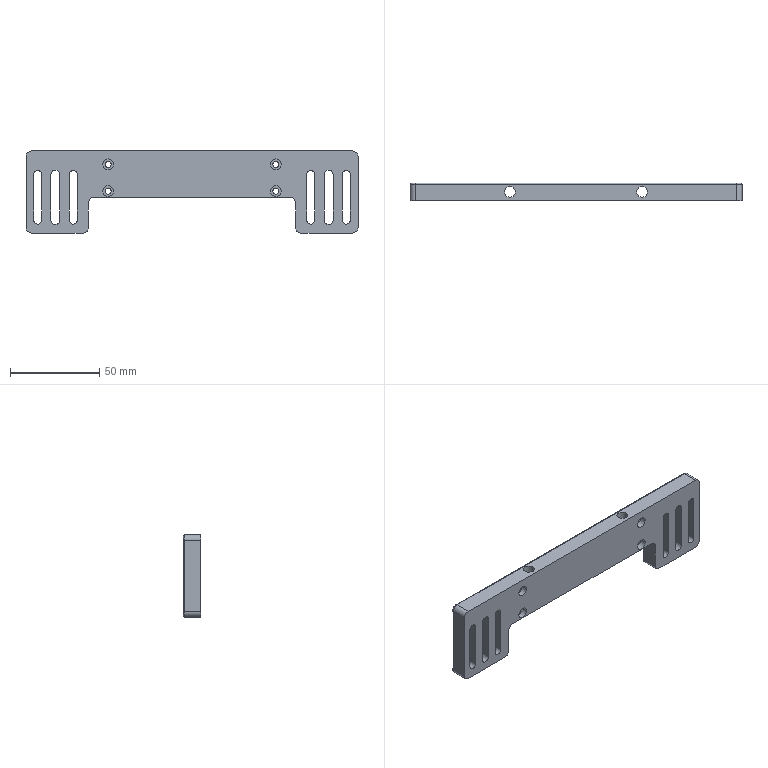Part | 1 solid | 90 faces | box 186 x 10 x 46 mm | volume 50794 mm3 | cylinder 46 | plane 36 | torus 8 | commonest cylinder face diameters 6 x12 2 x10 4.5 x8 3 x4 3.4 x4 5 x4